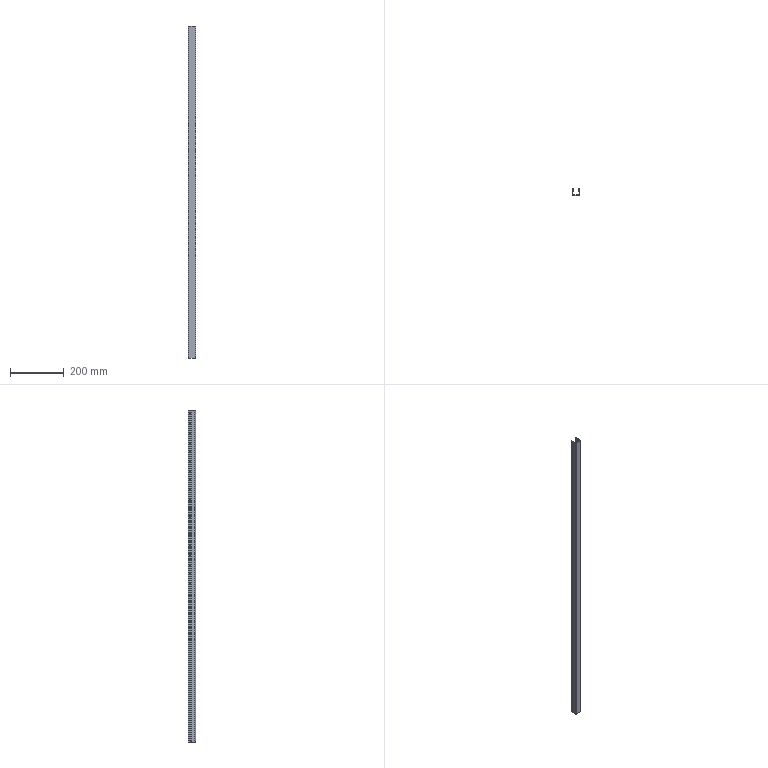Part | STEP file | Component2 | 1 solid | 120 faces | box 28.4 x 26.2 x 1238 mm | volume 123368 mm3 | cylinder 92 | plane 28 | commonest cylinder face diameters 4 x76 1.473 x8 3.873 x8